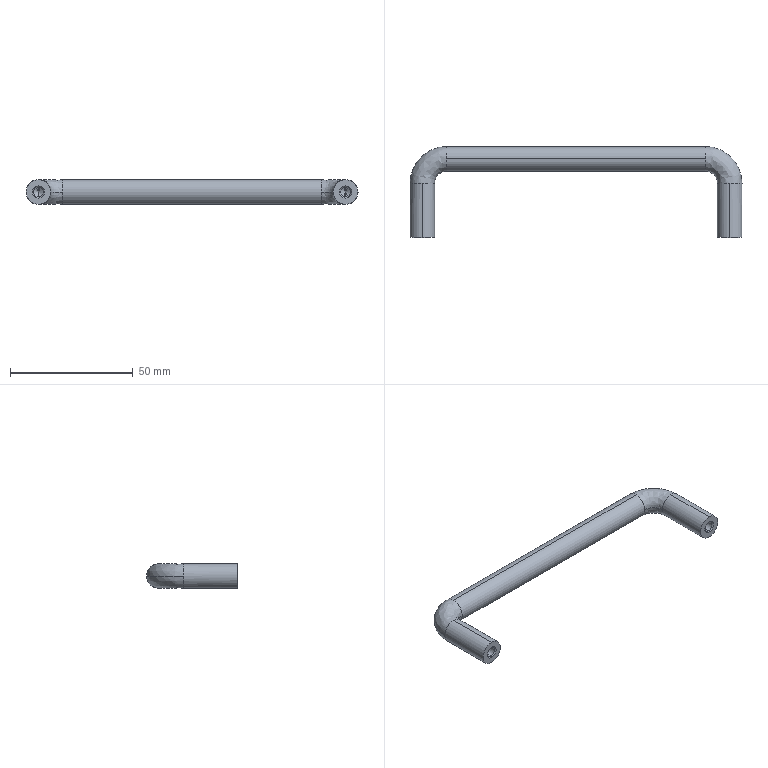Part | SolidWorks | features MBimport 1 | 1 solid | 24 faces | box 135 x 37 x 10 mm | volume 13834 mm3 | cylinder 10 | cone 8 | spline 4 | plane 2 | commonest cylinder face diameters 10 x6 4.134 x4
STEP:
#1=CARTESIAN_POINT('',(0.,13.193,0.));
#2=VERTEX_POINT('',#1);
#3=CARTESIAN_POINT('',(0.,12.,2.067));
#4=VERTEX_POINT('',#3);
#5=CARTESIAN_POINT('',(0.,12.,2.067));
#6=DIRECTION('',(0.,-0.5,0.866));
#7=VECTOR('',#6,1000.);
#8=LINE('',#5,#7);
#9=EDGE_CURVE('',#2,#4,#8,.T.);
#10=ORIENTED_EDGE('',*,*,#9,.F.);
#11=CARTESIAN_POINT('',(0.,12.,-2.067));
#12=VERTEX_POINT('',#11);
#13=CARTESIAN_POINT('',(0.,12.,-2.067));
#14=DIRECTION('',(0.,-0.5,-0.866));
#15=VECTOR('',#14,1000.);
#16=LINE('',#13,#15);
#17=EDGE_CURVE('',#2,#12,#16,.T.);
#18=ORIENTED_EDGE('',*,*,#17,.T.);
#19=CARTESIAN_POINT('',(0.,12.,0.));
#20=DIRECTION('',(0.,-1.,0.));
#21=DIRECTION('',(0.,0.,-1.));
#22=AXIS2_PLACEMENT_3D('',#19,#20,#21);
#23=CIRCLE('',#22,2.067);
#24=EDGE_CURVE('',#12,#4,#23,.T.);
#25=ORIENTED_EDGE('',*,*,#24,.T.);
#26=EDGE_LOOP('',(#10,#18,#25));
#27=FACE_OUTER_BOUND('',#26,.T.);
#28=CARTESIAN_POINT('',(0.,12.,0.));
#29=DIRECTION('',(0.,-1.,0.));
#30=DIRECTION('',(0.,0.,-1.));
#31=AXIS2_PLACEMENT_3D('',#28,#29,#30);
#32=CONICAL_SURFACE('',#31,2.067,1.047);
#33=ADVANCED_FACE('',(#27),#32,.F.);
#34=CARTESIAN_POINT('',(125.,13.193,0.));
#35=VERTEX_POINT('',#34);
#36=CARTESIAN_POINT('',(125.,12.,2.067));
#37=VERTEX_POINT('',#36);
#38=CARTESIAN_POINT('',(125.,12.,2.067));
#39=DIRECTION('',(0.,-0.5,0.866));
#40=VECTOR('',#39,1000.);
#41=LINE('',#38,#40);
#42=EDGE_CURVE('',#35,#37,#41,.T.);
#43=ORIENTED_EDGE('',*,*,#42,.F.);
#44=CARTESIAN_POINT('',(125.,12.,-2.067));
#45=VERTEX_POINT('',#44);
#46=CARTESIAN_POINT('',(125.,12.,-2.067));
#47=DIRECTION('',(0.,-0.5,-0.866));
#48=VECTOR('',#47,1000.);
#49=LINE('',#46,#48);
#50=EDGE_CURVE('',#35,#45,#49,.T.);
#51=ORIENTED_EDGE('',*,*,#50,.T.);
#52=CARTESIAN_POINT('',(125.,12.,0.));
#53=DIRECTION('',(0.,-1.,0.));
#54=DIRECTION('',(0.,0.,-1.));
#55=AXIS2_PLACEMENT_3D('',#52,#53,#54);
#56=CIRCLE('',#55,2.067);
#57=EDGE_CURVE('',#45,#37,#56,.T.);
#58=ORIENTED_EDGE('',*,*,#57,.T.);
#59=EDGE_LOOP('',(#43,#51,#58));
#60=FACE_OUTER_BOUND('',#59,.T.);
#61=CARTESIAN_POINT('',(125.,12.,0.));
#62=DIRECTION('',(0.,-1.,0.));
#63=DIRECTION('',(0.,0.,-1.));
#64=AXIS2_PLACEMENT_3D('',#61,#62,#63);
#65=CONICAL_SURFACE('',#64,2.067,1.047);
#66=ADVANCED_FACE('',(#60),#65,.F.);
#67=CARTESIAN_POINT('',(0.,0.433,2.067));
#68=VERTEX_POINT('',#67);
#69=CARTESIAN_POINT('',(0.,0.,2.067));
#70=DIRECTION('',(0.,-1.,0.));
#71=VECTOR('',#70,1000.);
#72=LINE('',#69,#71);
#73=EDGE_CURVE('',#4,#68,#72,.T.);
#74=ORIENTED_EDGE('',*,*,#73,.F.);
#75=ORIENTED_EDGE('',*,*,#24,.F.);
#76=CARTESIAN_POINT('',(0.,0.433,-2.067));
#77=VERTEX_POINT('',#76);
#78=CARTESIAN_POINT('',(0.,0.,-2.067));
#79=DIRECTION('',(0.,-1.,0.));
#80=VECTOR('',#79,1000.);
#81=LINE('',#78,#80);
#82=EDGE_CURVE('',#12,#77,#81,.T.);
#83=ORIENTED_EDGE('',*,*,#82,.T.);
#84=CARTESIAN_POINT('',(0.,0.433,0.));
#85=DIRECTION('',(0.,-1.,0.));
#86=DIRECTION('',(0.,0.,1.));
#87=AXIS2_PLACEMENT_3D('',#84,#85,#86);
#88=CIRCLE('',#87,2.067);
#89=EDGE_CURVE('',#77,#68,#88,.T.);
#90=ORIENTED_EDGE('',*,*,#89,.T.);
#91=EDGE_LOOP('',(#74,#75,#83,#90));
#92=FACE_OUTER_BOUND('',#91,.T.);
#93=CARTESIAN_POINT('',(0.,0.,0.));
#94=DIRECTION('',(0.,-1.,0.));
#95=DIRECTION('',(0.,0.,-1.));
#96=AXIS2_PLACEMENT_3D('',#93,#94,#95);
#97=CYLINDRICAL_SURFACE('',#96,2.067);
#98=ADVANCED_FACE('',(#92),#97,.F.);
#99=CARTESIAN_POINT('',(125.,0.433,2.067));
#100=VERTEX_POINT('',#99);
#101=CARTESIAN_POINT('',(125.,0.,2.067));
#102=DIRECTION('',(0.,-1.,0.));
#103=VECTOR('',#102,1000.);
#104=LINE('',#101,#103);
#105=EDGE_CURVE('',#37,#100,#104,.T.);
#106=ORIENTED_EDGE('',*,*,#105,.F.);
#107=ORIENTED_EDGE('',*,*,#57,.F.);
#108=CARTESIAN_POINT('',(125.,0.433,-2.067));
#109=VERTEX_POINT('',#108);
#110=CARTESIAN_POINT('',(125.,0.,-2.067));
#111=DIRECTION('',(0.,-1.,0.));
#112=VECTOR('',#111,1000.);
#113=LINE('',#110,#112);
#114=EDGE_CURVE('',#45,#109,#113,.T.);
#115=ORIENTED_EDGE('',*,*,#114,.T.);
#116=CARTESIAN_POINT('',(125.,0.433,0.));
#117=DIRECTION('',(0.,-1.,0.));
#118=DIRECTION('',(0.000000142,0.,1.));
#119=AXIS2_PLACEMENT_3D('',#116,#117,#118);
#120=CIRCLE('',#119,2.067);
#121=EDGE_CURVE('',#109,#100,#120,.T.);
#122=ORIENTED_EDGE('',*,*,#121,.T.);
#123=EDGE_LOOP('',(#106,#107,#115,#122));
#124=FACE_OUTER_BOUND('',#123,.T.);
#125=CARTESIAN_POINT('',(125.,0.,0.));
#126=DIRECTION('',(0.,-1.,0.));
#127=DIRECTION('',(0.,0.,-1.));
#128=AXIS2_PLACEMENT_3D('',#125,#126,#127);
#129=CYLINDRICAL_SURFACE('',#128,2.067);
#130=ADVANCED_FACE('',(#124),#129,.F.);
#131=CARTESIAN_POINT('',(0.,0.,2.5));
#132=VERTEX_POINT('',#131);
#133=CARTESIAN_POINT('',(0.,0.,2.5));
#134=DIRECTION('',(0.,-0.7071,0.7071));
#135=VECTOR('',#134,1000.);
#136=LINE('',#133,#135);
#137=EDGE_CURVE('',#68,#132,#136,.T.);
#138=ORIENTED_EDGE('',*,*,#137,.F.);
#139=ORIENTED_EDGE('',*,*,#89,.F.);
#140=CARTESIAN_POINT('',(0.,0.,-2.5));
#141=VERTEX_POINT('',#140);
#142=CARTESIAN_POINT('',(0.,0.,-2.5));
#143=DIRECTION('',(0.,-0.7071,-0.7071));
#144=VECTOR('',#143,1000.);
#145=LINE('',#142,#144);
#146=EDGE_CURVE('',#77,#141,#145,.T.);
#147=ORIENTED_EDGE('',*,*,#146,.T.);
#148=CARTESIAN_POINT('',(0.,0.,0.));
#149=DIRECTION('',(0.,1.,0.));
#150=DIRECTION('',(0.,0.,-1.));
#151=AXIS2_PLACEMENT_3D('',#148,#149,#150);
#152=CIRCLE('',#151,2.5);
#153=EDGE_CURVE('',#132,#141,#152,.T.);
#154=ORIENTED_EDGE('',*,*,#153,.F.);
#155=EDGE_LOOP('',(#138,#139,#147,#154));
#156=FACE_OUTER_BOUND('',#155,.T.);
#157=CARTESIAN_POINT('',(0.,0.,0.));
#158=DIRECTION('',(0.,-1.,0.));
#159=DIRECTION('',(0.,0.,-1.));
#160=AXIS2_PLACEMENT_3D('',#157,#158,#159);
#161=CONICAL_SURFACE('',#160,2.5,0.7854);
#162=ADVANCED_FACE('',(#156),#161,.F.);
#163=CARTESIAN_POINT('',(125.,0.,2.5));
#164=VERTEX_POINT('',#163);
#165=CARTESIAN_POINT('',(125.,0.,2.5));
#166=DIRECTION('',(0.,-0.7071,0.7071));
#167=VECTOR('',#166,1000.);
#168=LINE('',#165,#167);
#169=EDGE_CURVE('',#100,#164,#168,.T.);
#170=ORIENTED_EDGE('',*,*,#169,.F.);
#171=ORIENTED_EDGE('',*,*,#121,.F.);
#172=CARTESIAN_POINT('',(125.,0.,-2.5));
#173=VERTEX_POINT('',#172);
#174=CARTESIAN_POINT('',(125.,0.,-2.5));
#175=DIRECTION('',(0.,-0.7071,-0.7071));
#176=VECTOR('',#175,1000.);
#177=LINE('',#174,#176);
#178=EDGE_CURVE('',#109,#173,#177,.T.);
#179=ORIENTED_EDGE('',*,*,#178,.T.);
#180=CARTESIAN_POINT('',(125.,0.,0.));
#181=DIRECTION('',(0.,1.,0.));
#182=DIRECTION('',(0.,0.,-1.));
#183=AXIS2_PLACEMENT_3D('',#180,#181,#182);
#184=CIRCLE('',#183,2.5);
#185=EDGE_CURVE('',#164,#173,#184,.T.);
#186=ORIENTED_EDGE('',*,*,#185,.F.);
#187=EDGE_LOOP('',(#170,#171,#179,#186));
#188=FACE_OUTER_BOUND('',#187,.T.);
#189=CARTESIAN_POINT('',(125.,0.,0.));
#190=DIRECTION('',(0.,-1.,0.));
#191=DIRECTION('',(0.,0.,-1.));
#192=AXIS2_PLACEMENT_3D('',#189,#190,#191);
#193=CONICAL_SURFACE('',#192,2.5,0.7854);
#194=ADVANCED_FACE('',(#188),#193,.F.);
#195=CARTESIAN_POINT('',(0.,0.,0.));
#196=DIRECTION('',(0.,1.,0.));
#197=DIRECTION('',(0.,0.,-1.));
#198=AXIS2_PLACEMENT_3D('',#195,#196,#197);
#199=CIRCLE('',#198,2.5);
#200=EDGE_CURVE('',#141,#132,#199,.T.);
#201=ORIENTED_EDGE('',*,*,#200,.T.);
#202=ORIENTED_EDGE('',*,*,#153,.T.);
#203=EDGE_LOOP('',(#201,#202));
#204=FACE_BOUND('',#203,.T.);
#205=CARTESIAN_POINT('',(0.,0.,-5.));
#206=VERTEX_POINT('',#205);
#207=CARTESIAN_POINT('',(0.,0.,5.));
#208=VERTEX_POINT('',#207);
#209=CARTESIAN_POINT('',(0.,0.,0.));
#210=DIRECTION('',(0.,1.,0.));
#211=DIRECTION('',(0.,0.,-1.));
#212=AXIS2_PLACEMENT_3D('',#209,#210,#211);
#213=CIRCLE('',#212,5.);
#214=EDGE_CURVE('',#206,#208,#213,.T.);
#215=ORIENTED_EDGE('',*,*,#214,.F.);
#216=CARTESIAN_POINT('',(0.,0.,0.));
#217=DIRECTION('',(0.,1.,0.));
#218=DIRECTION('',(0.,0.,-1.));
#219=AXIS2_PLACEMENT_3D('',#216,#217,#218);
#220=CIRCLE('',#219,5.);
#221=EDGE_CURVE('',#208,#206,#220,.T.);
#222=ORIENTED_EDGE('',*,*,#221,.F.);
#223=EDGE_LOOP('',(#215,#222));
#224=FACE_OUTER_BOUND('',#223,.T.);
#225=CARTESIAN_POINT('',(-5.,0.,-5.));
#226=DIRECTION('',(0.,-1.,0.));
#227=DIRECTION('',(0.,0.,-1.));
#228=AXIS2_PLACEMENT_3D('',#225,#226,#227);
#229=PLANE('',#228);
#230=ADVANCED_FACE('',(#204,#224),#229,.T.);
#231=CARTESIAN_POINT('',(125.,0.,0.));
#232=DIRECTION('',(0.,1.,0.));
#233=DIRECTION('',(0.,0.,-1.));
#234=AXIS2_PLACEMENT_3D('',#231,#232,#233);
#235=CIRCLE('',#234,2.5);
#236=EDGE_CURVE('',#173,#164,#235,.T.);
#237=ORIENTED_EDGE('',*,*,#236,.T.);
#238=ORIENTED_EDGE('',*,*,#185,.T.);
#239=EDGE_LOOP('',(#237,#238));
#240=FACE_BOUND('',#239,.T.);
#241=CARTESIAN_POINT('',(125.,0.,-5.));
#242=VERTEX_POINT('',#241);
#243=CARTESIAN_POINT('',(125.,0.,5.));
#244=VERTEX_POINT('',#243);
#245=CARTESIAN_POINT('',(125.,0.,0.));
#246=DIRECTION('',(0.,1.,0.));
#247=DIRECTION('',(0.,0.,-1.));
#248=AXIS2_PLACEMENT_3D('',#245,#246,#247);
#249=CIRCLE('',#248,5.);
#250=EDGE_CURVE('',#242,#244,#249,.T.);
#251=ORIENTED_EDGE('',*,*,#250,.F.);
#252=CARTESIAN_POINT('',(125.,0.,0.));
#253=DIRECTION('',(0.,1.,0.));
#254=DIRECTION('',(0.,0.,-1.));
#255=AXIS2_PLACEMENT_3D('',#252,#253,#254);
#256=CIRCLE('',#255,5.);
#257=EDGE_CURVE('',#244,#242,#256,.T.);
#258=ORIENTED_EDGE('',*,*,#257,.F.);
#259=EDGE_LOOP('',(#251,#258));
#260=FACE_OUTER_BOUND('',#259,.T.);
#261=CARTESIAN_POINT('',(120.,0.,-5.));
#262=DIRECTION('',(0.,-1.,0.));
#263=DIRECTION('',(0.,0.,-1.));
#264=AXIS2_PLACEMENT_3D('',#261,#262,#263);
#265=PLANE('',#264);
#266=ADVANCED_FACE('',(#240,#260),#265,.T.);
#267=CARTESIAN_POINT('',(0.,22.,5.));
#268=VERTEX_POINT('',#267);
#269=CARTESIAN_POINT('',(0.,0.,5.));
#270=DIRECTION('',(0.,-1.,0.));
#271=VECTOR('',#270,1000.);
#272=LINE('',#269,#271);
#273=EDGE_CURVE('',#268,#208,#272,.T.);
#274=ORIENTED_EDGE('',*,*,#273,.F.);
#275=CARTESIAN_POINT('',(-5.,22.,0.));
#276=VERTEX_POINT('',#275);
#277=CARTESIAN_POINT('',(0.,22.,0.));
#278=DIRECTION('',(0.,1.,0.));
#279=DIRECTION('',(-1.,0.,0.));
#280=AXIS2_PLACEMENT_3D('',#277,#278,#279);
#281=CIRCLE('',#280,5.);
#282=EDGE_CURVE('',#276,#268,#281,.T.);
#283=ORIENTED_EDGE('',*,*,#282,.F.);
#284=CARTESIAN_POINT('',(0.,22.,-5.));
#285=VERTEX_POINT('',#284);
#286=CARTESIAN_POINT('',(0.,22.,0.));
#287=DIRECTION('',(0.,1.,0.));
#288=DIRECTION('',(-1.,0.,0.));
#289=AXIS2_PLACEMENT_3D('',#286,#287,#288);
#290=CIRCLE('',#289,5.);
#291=EDGE_CURVE('',#285,#276,#290,.T.);
#292=ORIENTED_EDGE('',*,*,#291,.F.);
#293=CARTESIAN_POINT('',(0.,0.,-5.));
#294=DIRECTION('',(0.,-1.,0.));
#295=VECTOR('',#294,1000.);
#296=LINE('',#293,#295);
#297=EDGE_CURVE('',#285,#206,#296,.T.);
#298=ORIENTED_EDGE('',*,*,#297,.T.);
#299=ORIENTED_EDGE('',*,*,#214,.T.);
#300=EDGE_LOOP('',(#274,#283,#292,#298,#299));
#301=FACE_OUTER_BOUND('',#300,.T.);
#302=CARTESIAN_POINT('',(0.,0.,0.));
#303=DIRECTION('',(0.,-1.,0.));
#304=DIRECTION('',(0.,0.,-1.));
#305=AXIS2_PLACEMENT_3D('',#302,#303,#304);
#306=CYLINDRICAL_SURFACE('',#305,5.);
#307=ADVANCED_FACE('',(#301),#306,.T.);
#308=CARTESIAN_POINT('',(125.,22.,5.));
#309=VERTEX_POINT('',#308);
#310=CARTESIAN_POINT('',(125.,0.,5.));
#311=DIRECTION('',(0.,-1.,0.));
#312=VECTOR('',#311,1000.);
#313=LINE('',#310,#312);
#314=EDGE_CURVE('',#309,#244,#313,.T.);
#315=ORIENTED_EDGE('',*,*,#314,.F.);
#316=CARTESIAN_POINT('',(120.,22.,0.));
#317=VERTEX_POINT('',#316);
#318=CARTESIAN_POINT('',(125.,22.,0.));
#319=DIRECTION('',(0.,1.,0.));
#320=DIRECTION('',(1.,0.,0.));
#321=AXIS2_PLACEMENT_3D('',#318,#319,#320);
#322=CIRCLE('',#321,5.);
#323=EDGE_CURVE('',#317,#309,#322,.T.);
#324=ORIENTED_EDGE('',*,*,#323,.F.);
#325=CARTESIAN_POINT('',(125.,22.,-5.));
#326=VERTEX_POINT('',#325);
#327=CARTESIAN_POINT('',(125.,22.,0.));
#328=DIRECTION('',(0.,1.,0.));
#329=DIRECTION('',(1.,0.,0.));
#330=AXIS2_PLACEMENT_3D('',#327,#328,#329);
#331=CIRCLE('',#330,5.);
#332=EDGE_CURVE('',#326,#317,#331,.T.);
#333=ORIENTED_EDGE('',*,*,#332,.F.);
#334=CARTESIAN_POINT('',(125.,0.,-5.));
#335=DIRECTION('',(0.,-1.,0.));
#336=VECTOR('',#335,1000.);
#337=LINE('',#334,#336);
#338=EDGE_CURVE('',#326,#242,#337,.T.);
#339=ORIENTED_EDGE('',*,*,#338,.T.);
#340=ORIENTED_EDGE('',*,*,#250,.T.);
#341=EDGE_LOOP('',(#315,#324,#333,#339,#340));
#342=FACE_OUTER_BOUND('',#341,.T.);
#343=CARTESIAN_POINT('',(125.,0.,0.));
#344=DIRECTION('',(0.,-1.,0.));
#345=DIRECTION('',(0.,0.,-1.));
#346=AXIS2_PLACEMENT_3D('',#343,#344,#345);
#347=CYLINDRICAL_SURFACE('',#346,5.);
#348=ADVANCED_FACE('',(#342),#347,.T.);
#349=CARTESIAN_POINT('',(5.,22.,0.));
#350=VERTEX_POINT('',#349);
#351=CARTESIAN_POINT('',(10.,27.,0.));
#352=VERTEX_POINT('',#351);
#353=CARTESIAN_POINT('',(10.,22.,0.));
#354=DIRECTION('',(0.,0.,-1.));
#355=DIRECTION('',(-1.,0.,0.));
#356=AXIS2_PLACEMENT_3D('',#353,#354,#355);
#357=CIRCLE('',#356,5.);
#358=EDGE_CURVE('',#350,#352,#357,.T.);
#359=ORIENTED_EDGE('',*,*,#358,.F.);
#360=CARTESIAN_POINT('',(0.,22.,0.));
#361=DIRECTION('',(0.,1.,0.));
#362=DIRECTION('',(-1.,0.,0.));
#363=AXIS2_PLACEMENT_3D('',#360,#361,#362);
#364=CIRCLE('',#363,5.);
#365=EDGE_CURVE('',#350,#285,#364,.T.);
#366=ORIENTED_EDGE('',*,*,#365,.T.);
#367=ORIENTED_EDGE('',*,*,#291,.T.);
#368=CARTESIAN_POINT('',(10.,37.,0.));
#369=VERTEX_POINT('',#368);
#370=CARTESIAN_POINT('',(10.,22.,0.));
#371=DIRECTION('',(0.,0.,-1.));
#372=DIRECTION('',(-1.,0.,0.));
#373=AXIS2_PLACEMENT_3D('',#370,#371,#372);
#374=CIRCLE('',#373,15.);
#375=EDGE_CURVE('',#276,#369,#374,.T.);
#376=ORIENTED_EDGE('',*,*,#375,.T.);
#377=CARTESIAN_POINT('',(10.,32.,-5.));
#378=VERTEX_POINT('',#377);
#379=CARTESIAN_POINT('',(10.,32.,0.));
#380=DIRECTION('',(1.,0.,0.));
#381=DIRECTION('',(0.,0.,-1.));
#382=AXIS2_PLACEMENT_3D('',#379,#380,#381);
#383=CIRCLE('',#382,5.);
#384=EDGE_CURVE('',#378,#369,#383,.T.);
#385=ORIENTED_EDGE('',*,*,#384,.F.);
#386=CARTESIAN_POINT('',(10.,32.,0.));
#387=DIRECTION('',(1.,0.,0.));
#388=DIRECTION('',(0.,0.,-1.));
#389=AXIS2_PLACEMENT_3D('',#386,#387,#388);
#390=CIRCLE('',#389,5.);
#391=EDGE_CURVE('',#352,#378,#390,.T.);
#392=ORIENTED_EDGE('',*,*,#391,.F.);
#393=EDGE_LOOP('',(#359,#366,#367,#376,#385,#392));
#394=FACE_OUTER_BOUND('',#393,.T.);
#395=CARTESIAN_POINT('',(5.,22.,0.));
#396=CARTESIAN_POINT('',(5.,24.929,0.));
#397=CARTESIAN_POINT('',(7.071,27.,0.));
#398=CARTESIAN_POINT('',(10.,27.,0.));
#399=CARTESIAN_POINT('',(5.,22.,-10.));
#400=CARTESIAN_POINT('',(5.,24.929,-10.));
#401=CARTESIAN_POINT('',(7.071,27.,-10.));
#402=CARTESIAN_POINT('',(10.,27.,-10.));
#403=CARTESIAN_POINT('',(-5.,22.,-10.));
#404=CARTESIAN_POINT('',(-5.,30.787,-10.));
#405=CARTESIAN_POINT('',(1.213,37.,-10.));
#406=CARTESIAN_POINT('',(10.,37.,-10.));
#407=CARTESIAN_POINT('',(-5.,22.,0.));
#408=CARTESIAN_POINT('',(-5.,30.787,0.));
#409=CARTESIAN_POINT('',(1.213,37.,0.));
#410=CARTESIAN_POINT('',(10.,37.,0.));
#411=(BOUNDED_SURFACE()B_SPLINE_SURFACE(3,3,((#395,#396,#397,#398),(#399,#400,#401,#402),(#403,#404,#405,#406),(#407,#408,#409,#410)),.UNSPECIFIED.,.F.,.F.,.F.)B_SPLINE_SURFACE_WITH_KNOTS((4,4),(4,4),(0.,1.),(0.,1.),.UNSPECIFIED.)GEOMETRIC_REPRESENTATION_ITEM()RATIONAL_B_SPLINE_SURFACE(((1.,0.8047,0.8047,1.),(0.3333,0.2682,0.2682,0.3333),(0.3333,0.2682,0.2682,0.3333),(1.,0.8047,0.8047,1.)))REPRESENTATION_ITEM('')SURFACE());
#412=ADVANCED_FACE('',(#394),#411,.T.);
#413=CARTESIAN_POINT('',(115.,27.,0.));
#414=VERTEX_POINT('',#413);
#415=CARTESIAN_POINT('',(115.,22.,0.));
#416=DIRECTION('',(0.,0.,1.));
#417=DIRECTION('',(1.,0.,0.));
#418=AXIS2_PLACEMENT_3D('',#415,#416,#417);
#419=CIRCLE('',#418,5.);
#420=EDGE_CURVE('',#317,#414,#419,.T.);
#421=ORIENTED_EDGE('',*,*,#420,.F.);
#422=ORIENTED_EDGE('',*,*,#323,.T.);
#423=CARTESIAN_POINT('',(130.,22.,0.));
#424=VERTEX_POINT('',#423);
#425=CARTESIAN_POINT('',(125.,22.,0.));
#426=DIRECTION('',(0.,1.,0.));
#427=DIRECTION('',(1.,0.,0.));
#428=AXIS2_PLACEMENT_3D('',#425,#426,#427);
#429=CIRCLE('',#428,5.);
#430=EDGE_CURVE('',#309,#424,#429,.T.);
#431=ORIENTED_EDGE('',*,*,#430,.T.);
#432=CARTESIAN_POINT('',(115.,37.,0.));
#433=VERTEX_POINT('',#432);
#434=CARTESIAN_POINT('',(115.,22.,0.));
#435=DIRECTION('',(0.,0.,1.));
#436=DIRECTION('',(1.,0.,0.));
#437=AXIS2_PLACEMENT_3D('',#434,#435,#436);
#438=CIRCLE('',#437,15.);
#439=EDGE_CURVE('',#424,#433,#438,.T.);
#440=ORIENTED_EDGE('',*,*,#439,.T.);
#441=CARTESIAN_POINT('',(115.,32.,5.));
#442=VERTEX_POINT('',#441);
#443=CARTESIAN_POINT('',(115.,32.,0.));
#444=DIRECTION('',(-1.,0.,0.));
#445=DIRECTION('',(0.,0.,-1.));
#446=AXIS2_PLACEMENT_3D('',#443,#444,#445);
#447=CIRCLE('',#446,5.);
#448=EDGE_CURVE('',#442,#433,#447,.T.);
#449=ORIENTED_EDGE('',*,*,#448,.F.);
#450=CARTESIAN_POINT('',(115.,32.,0.));
#451=DIRECTION('',(-1.,0.,0.));
#452=DIRECTION('',(0.,0.,-1.));
#453=AXIS2_PLACEMENT_3D('',#450,#451,#452);
#454=CIRCLE('',#453,5.);
#455=EDGE_CURVE('',#414,#442,#454,.T.);
#456=ORIENTED_EDGE('',*,*,#455,.F.);
#457=EDGE_LOOP('',(#421,#422,#431,#440,#449,#456));
#458=FACE_OUTER_BOUND('',#457,.T.);
#459=CARTESIAN_POINT('',(120.,22.,0.));
#460=CARTESIAN_POINT('',(120.,24.929,0.));
#461=CARTESIAN_POINT('',(117.929,27.,0.));
#462=CARTESIAN_POINT('',(115.,27.,0.));
#463=CARTESIAN_POINT('',(120.,22.,10.));
#464=CARTESIAN_POINT('',(120.,24.929,10.));
#465=CARTESIAN_POINT('',(117.929,27.,10.));
#466=CARTESIAN_POINT('',(115.,27.,10.));
#467=CARTESIAN_POINT('',(130.,22.,10.));
#468=CARTESIAN_POINT('',(130.,30.787,10.));
#469=CARTESIAN_POINT('',(123.787,37.,10.));
#470=CARTESIAN_POINT('',(115.,37.,10.));
#471=CARTESIAN_POINT('',(130.,22.,0.));
#472=CARTESIAN_POINT('',(130.,30.787,0.));
#473=CARTESIAN_POINT('',(123.787,37.,0.));
#474=CARTESIAN_POINT('',(115.,37.,0.));
#475=(BOUNDED_SURFACE()B_SPLINE_SURFACE(3,3,((#459,#460,#461,#462),(#463,#464,#465,#466),(#467,#468,#469,#470),(#471,#472,#473,#474)),.UNSPECIFIED.,.F.,.F.,.F.)B_SPLINE_SURFACE_WITH_KNOTS((4,4),(4,4),(0.,1.),(0.,1.),.UNSPECIFIED.)GEOMETRIC_REPRESENTATION_ITEM()RATIONAL_B_SPLINE_SURFACE(((1.,0.8047,0.8047,1.),(0.3333,0.2682,0.2682,0.3333),(0.3333,0.2682,0.2682,0.3333),(1.,0.8047,0.8047,1.)))REPRESENTATION_ITEM('')SURFACE());
#476=ADVANCED_FACE('',(#458),#475,.T.);
#477=CARTESIAN_POINT('',(10.,32.,5.));
#478=VERTEX_POINT('',#477);
#479=CARTESIAN_POINT('',(70.,32.,5.));
#480=DIRECTION('',(1.,0.,0.));
#481=VECTOR('',#480,1000.);
#482=LINE('',#479,#481);
#483=EDGE_CURVE('',#478,#442,#482,.T.);
#484=ORIENTED_EDGE('',*,*,#483,.F.);
#485=CARTESIAN_POINT('',(10.,32.,0.));
#486=DIRECTION('',(1.,0.,0.));
#487=DIRECTION('',(0.,0.,-1.));
#488=AXIS2_PLACEMENT_3D('',#485,#486,#487);
#489=CIRCLE('',#488,5.);
#490=EDGE_CURVE('',#478,#352,#489,.T.);
#491=ORIENTED_EDGE('',*,*,#490,.T.);
#492=ORIENTED_EDGE('',*,*,#391,.T.);
#493=CARTESIAN_POINT('',(115.,32.,-5.));
#494=VERTEX_POINT('',#493);
#495=CARTESIAN_POINT('',(70.,32.,-5.));
#496=DIRECTION('',(1.,0.,0.));
#497=VECTOR('',#496,1000.);
#498=LINE('',#495,#497);
#499=EDGE_CURVE('',#378,#494,#498,.T.);
#500=ORIENTED_EDGE('',*,*,#499,.T.);
#501=CARTESIAN_POINT('',(115.,32.,0.));
#502=DIRECTION('',(-1.,0.,0.));
#503=DIRECTION('',(0.,0.,-1.));
#504=AXIS2_PLACEMENT_3D('',#501,#502,#503);
#505=CIRCLE('',#504,5.);
#506=EDGE_CURVE('',#494,#414,#505,.T.);
#507=ORIENTED_EDGE('',*,*,#506,.T.);
#508=ORIENTED_EDGE('',*,*,#455,.T.);
#509=EDGE_LOOP('',(#484,#491,#492,#500,#507,#508));
#510=FACE_OUTER_BOUND('',#509,.T.);
#511=CARTESIAN_POINT('',(70.,32.,0.));
#512=DIRECTION('',(1.,0.,0.));
#513=DIRECTION('',(0.,0.,-1.));
#514=AXIS2_PLACEMENT_3D('',#511,#512,#513);
#515=CYLINDRICAL_SURFACE('',#514,5.);
#516=ADVANCED_FACE('',(#510),#515,.T.);
#517=ORIENTED_EDGE('',*,*,#17,.F.);
#518=ORIENTED_EDGE('',*,*,#9,.T.);
#519=CARTESIAN_POINT('',(0.,12.,0.));
#520=DIRECTION('',(0.,-1.,0.));
#521=DIRECTION('',(0.,0.,-1.));
#522=AXIS2_PLACEMENT_3D('',#519,#520,#521);
#523=CIRCLE('',#522,2.067);
#524=EDGE_CURVE('',#4,#12,#523,.T.);
#525=ORIENTED_EDGE('',*,*,#524,.T.);
#526=EDGE_LOOP('',(#517,#518,#525));
#527=FACE_OUTER_BOUND('',#526,.T.);
#528=CARTESIAN_POINT('',(0.,12.,0.));
#529=DIRECTION('',(0.,-1.,0.));
#530=DIRECTION('',(0.,0.,-1.));
#531=AXIS2_PLACEMENT_3D('',#528,#529,#530);
#532=CONICAL_SURFACE('',#531,2.067,1.047);
#533=ADVANCED_FACE('',(#527),#532,.F.);
#534=ORIENTED_EDGE('',*,*,#50,.F.);
#535=ORIENTED_EDGE('',*,*,#42,.T.);
#536=CARTESIAN_POINT('',(125.,12.,0.));
#537=DIRECTION('',(0.,-1.,0.));
#538=DIRECTION('',(0.,0.,-1.));
#539=AXIS2_PLACEMENT_3D('',#536,#537,#538);
#540=CIRCLE('',#539,2.067);
#541=EDGE_CURVE('',#37,#45,#540,.T.);
#542=ORIENTED_EDGE('',*,*,#541,.T.);
#543=EDGE_LOOP('',(#534,#535,#542));
#544=FACE_OUTER_BOUND('',#543,.T.);
#545=CARTESIAN_POINT('',(125.,12.,0.));
#546=DIRECTION('',(0.,-1.,0.));
#547=DIRECTION('',(0.,0.,-1.));
#548=AXIS2_PLACEMENT_3D('',#545,#546,#547);
#549=CONICAL_SURFACE('',#548,2.067,1.047);
#550=ADVANCED_FACE('',(#544),#549,.F.);
#551=ORIENTED_EDGE('',*,*,#524,.F.);
#552=ORIENTED_EDGE('',*,*,#73,.T.);
#553=CARTESIAN_POINT('',(0.,0.433,0.));
#554=DIRECTION('',(0.,-1.,0.));
#555=DIRECTION('',(0.,0.,1.));
#556=AXIS2_PLACEMENT_3D('',#553,#554,#555);
#557=CIRCLE('',#556,2.067);
#558=EDGE_CURVE('',#68,#77,#557,.T.);
#559=ORIENTED_EDGE('',*,*,#558,.T.);
#560=ORIENTED_EDGE('',*,*,#82,.F.);
#561=EDGE_LOOP('',(#551,#552,#559,#560));
#562=FACE_OUTER_BOUND('',#561,.T.);
#563=CARTESIAN_POINT('',(0.,0.,0.));
#564=DIRECTION('',(0.,-1.,0.));
#565=DIRECTION('',(0.,0.,-1.));
#566=AXIS2_PLACEMENT_3D('',#563,#564,#565);
#567=CYLINDRICAL_SURFACE('',#566,2.067);
#568=ADVANCED_FACE('',(#562),#567,.F.);
#569=ORIENTED_EDGE('',*,*,#541,.F.);
#570=ORIENTED_EDGE('',*,*,#105,.T.);
#571=CARTESIAN_POINT('',(125.,0.433,0.));
#572=DIRECTION('',(0.,-1.,0.));
#573=DIRECTION('',(0.000000142,0.,1.));
#574=AXIS2_PLACEMENT_3D('',#571,#572,#573);
#575=CIRCLE('',#574,2.067);
#576=EDGE_CURVE('',#100,#109,#575,.T.);
#577=ORIENTED_EDGE('',*,*,#576,.T.);
#578=ORIENTED_EDGE('',*,*,#114,.F.);
#579=EDGE_LOOP('',(#569,#570,#577,#578));
#580=FACE_OUTER_BOUND('',#579,.T.);
#581=CARTESIAN_POINT('',(125.,0.,0.));
#582=DIRECTION('',(0.,-1.,0.));
#583=DIRECTION('',(0.,0.,-1.));
#584=AXIS2_PLACEMENT_3D('',#581,#582,#583);
#585=CYLINDRICAL_SURFACE('',#584,2.067);
#586=ADVANCED_FACE('',(#580),#585,.F.);
#587=ORIENTED_EDGE('',*,*,#558,.F.);
#588=ORIENTED_EDGE('',*,*,#137,.T.);
#589=ORIENTED_EDGE('',*,*,#200,.F.);
#590=ORIENTED_EDGE('',*,*,#146,.F.);
#591=EDGE_LOOP('',(#587,#588,#589,#590));
#592=FACE_OUTER_BOUND('',#591,.T.);
#593=CARTESIAN_POINT('',(0.,0.,0.));
#594=DIRECTION('',(0.,-1.,0.));
#595=DIRECTION('',(0.,0.,-1.));
#596=AXIS2_PLACEMENT_3D('',#593,#594,#595);
#597=CONICAL_SURFACE('',#596,2.5,0.7854);
#598=ADVANCED_FACE('',(#592),#597,.F.);
#599=ORIENTED_EDGE('',*,*,#576,.F.);
#600=ORIENTED_EDGE('',*,*,#169,.T.);
#601=ORIENTED_EDGE('',*,*,#236,.F.);
#602=ORIENTED_EDGE('',*,*,#178,.F.);
#603=EDGE_LOOP('',(#599,#600,#601,#602));
#604=FACE_OUTER_BOUND('',#603,.T.);
#605=CARTESIAN_POINT('',(125.,0.,0.));
#606=DIRECTION('',(0.,-1.,0.));
#607=DIRECTION('',(0.,0.,-1.));
#608=AXIS2_PLACEMENT_3D('',#605,#606,#607);
#609=CONICAL_SURFACE('',#608,2.5,0.7854);
#610=ADVANCED_FACE('',(#604),#609,.F.);
#611=CARTESIAN_POINT('',(0.,22.,0.));
#612=DIRECTION('',(0.,1.,0.));
#613=DIRECTION('',(-1.,0.,0.));
#614=AXIS2_PLACEMENT_3D('',#611,#612,#613);
#615=CIRCLE('',#614,5.);
#616=EDGE_CURVE('',#268,#350,#615,.T.);
#617=ORIENTED_EDGE('',*,*,#616,.F.);
#618=ORIENTED_EDGE('',*,*,#273,.T.);
#619=ORIENTED_EDGE('',*,*,#221,.T.);
#620=ORIENTED_EDGE('',*,*,#297,.F.);
#621=ORIENTED_EDGE('',*,*,#365,.F.);
#622=EDGE_LOOP('',(#617,#618,#619,#620,#621));
#623=FACE_OUTER_BOUND('',#622,.T.);
#624=CARTESIAN_POINT('',(0.,0.,0.));
#625=DIRECTION('',(0.,-1.,0.));
#626=DIRECTION('',(0.,0.,-1.));
#627=AXIS2_PLACEMENT_3D('',#624,#625,#626);
#628=CYLINDRICAL_SURFACE('',#627,5.);
#629=ADVANCED_FACE('',(#623),#628,.T.);
#630=ORIENTED_EDGE('',*,*,#430,.F.);
#631=ORIENTED_EDGE('',*,*,#314,.T.);
#632=ORIENTED_EDGE('',*,*,#257,.T.);
#633=ORIENTED_EDGE('',*,*,#338,.F.);
#634=CARTESIAN_POINT('',(125.,22.,0.));
#635=DIRECTION('',(0.,1.,0.));
#636=DIRECTION('',(1.,0.,0.));
#637=AXIS2_PLACEMENT_3D('',#634,#635,#636);
#638=CIRCLE('',#637,5.);
#639=EDGE_CURVE('',#424,#326,#638,.T.);
#640=ORIENTED_EDGE('',*,*,#639,.F.);
#641=EDGE_LOOP('',(#630,#631,#632,#633,#640));
#642=FACE_OUTER_BOUND('',#641,.T.);
#643=CARTESIAN_POINT('',(125.,0.,0.));
#644=DIRECTION('',(0.,-1.,0.));
#645=DIRECTION('',(0.,0.,-1.));
#646=AXIS2_PLACEMENT_3D('',#643,#644,#645);
#647=CYLINDRICAL_SURFACE('',#646,5.);
#648=ADVANCED_FACE('',(#642),#647,.T.);
#649=ORIENTED_EDGE('',*,*,#616,.T.);
#650=ORIENTED_EDGE('',*,*,#358,.T.);
#651=ORIENTED_EDGE('',*,*,#490,.F.);
#652=CARTESIAN_POINT('',(10.,32.,0.));
#653=DIRECTION('',(1.,0.,0.));
#654=DIRECTION('',(0.,0.,-1.));
#655=AXIS2_PLACEMENT_3D('',#652,#653,#654);
#656=CIRCLE('',#655,5.);
#657=EDGE_CURVE('',#369,#478,#656,.T.);
#658=ORIENTED_EDGE('',*,*,#657,.F.);
#659=ORIENTED_EDGE('',*,*,#375,.F.);
#660=ORIENTED_EDGE('',*,*,#282,.T.);
#661=EDGE_LOOP('',(#649,#650,#651,#658,#659,#660));
#662=FACE_OUTER_BOUND('',#661,.T.);
#663=CARTESIAN_POINT('',(-5.,22.,0.));
#664=CARTESIAN_POINT('',(-5.,30.787,0.));
#665=CARTESIAN_POINT('',(1.213,37.,0.));
#666=CARTESIAN_POINT('',(10.,37.,0.));
#667=CARTESIAN_POINT('',(-5.,22.,10.));
#668=CARTESIAN_POINT('',(-5.,30.787,10.));
#669=CARTESIAN_POINT('',(1.213,37.,10.));
#670=CARTESIAN_POINT('',(10.,37.,10.));
#671=CARTESIAN_POINT('',(5.,22.,10.));
#672=CARTESIAN_POINT('',(5.,24.929,10.));
#673=CARTESIAN_POINT('',(7.071,27.,10.));
#674=CARTESIAN_POINT('',(10.,27.,10.));
#675=CARTESIAN_POINT('',(5.,22.,0.));
#676=CARTESIAN_POINT('',(5.,24.929,0.));
#677=CARTESIAN_POINT('',(7.071,27.,0.));
#678=CARTESIAN_POINT('',(10.,27.,0.));
#679=(BOUNDED_SURFACE()B_SPLINE_SURFACE(3,3,((#663,#664,#665,#666),(#667,#668,#669,#670),(#671,#672,#673,#674),(#675,#676,#677,#678)),.UNSPECIFIED.,.F.,.F.,.T.)B_SPLINE_SURFACE_WITH_KNOTS((4,4),(4,4),(0.,1.),(0.,1.),.UNSPECIFIED.)GEOMETRIC_REPRESENTATION_ITEM()RATIONAL_B_SPLINE_SURFACE(((1.,0.8047,0.8047,1.),(0.3333,0.2682,0.2682,0.3333),(0.3333,0.2682,0.2682,0.3333),(1.,0.8047,0.8047,1.)))REPRESENTATION_ITEM('')SURFACE());
#680=ADVANCED_FACE('',(#662),#679,.T.);
#681=ORIENTED_EDGE('',*,*,#332,.T.);
#682=ORIENTED_EDGE('',*,*,#420,.T.);
#683=ORIENTED_EDGE('',*,*,#506,.F.);
#684=CARTESIAN_POINT('',(115.,32.,0.));
#685=DIRECTION('',(-1.,0.,0.));
#686=DIRECTION('',(0.,0.,-1.));
#687=AXIS2_PLACEMENT_3D('',#684,#685,#686);
#688=CIRCLE('',#687,5.);
#689=EDGE_CURVE('',#433,#494,#688,.T.);
#690=ORIENTED_EDGE('',*,*,#689,.F.);
#691=ORIENTED_EDGE('',*,*,#439,.F.);
#692=ORIENTED_EDGE('',*,*,#639,.T.);
#693=EDGE_LOOP('',(#681,#682,#683,#690,#691,#692));
#694=FACE_OUTER_BOUND('',#693,.T.);
#695=CARTESIAN_POINT('',(130.,22.,0.));
#696=CARTESIAN_POINT('',(130.,30.787,0.));
#697=CARTESIAN_POINT('',(123.787,37.,0.));
#698=CARTESIAN_POINT('',(115.,37.,0.));
#699=CARTESIAN_POINT('',(130.,22.,-10.));
#700=CARTESIAN_POINT('',(130.,30.787,-10.));
#701=CARTESIAN_POINT('',(123.787,37.,-10.));
#702=CARTESIAN_POINT('',(115.,37.,-10.));
#703=CARTESIAN_POINT('',(120.,22.,-10.));
#704=CARTESIAN_POINT('',(120.,24.929,-10.));
#705=CARTESIAN_POINT('',(117.929,27.,-10.));
#706=CARTESIAN_POINT('',(115.,27.,-10.));
#707=CARTESIAN_POINT('',(120.,22.,0.));
#708=CARTESIAN_POINT('',(120.,24.929,0.));
#709=CARTESIAN_POINT('',(117.929,27.,0.));
#710=CARTESIAN_POINT('',(115.,27.,0.));
#711=(BOUNDED_SURFACE()B_SPLINE_SURFACE(3,3,((#695,#696,#697,#698),(#699,#700,#701,#702),(#703,#704,#705,#706),(#707,#708,#709,#710)),.UNSPECIFIED.,.F.,.F.,.T.)B_SPLINE_SURFACE_WITH_KNOTS((4,4),(4,4),(0.,1.),(0.,1.),.UNSPECIFIED.)GEOMETRIC_REPRESENTATION_ITEM()RATIONAL_B_SPLINE_SURFACE(((1.,0.8047,0.8047,1.),(0.3333,0.2682,0.2682,0.3333),(0.3333,0.2682,0.2682,0.3333),(1.,0.8047,0.8047,1.)))REPRESENTATION_ITEM('')SURFACE());
#712=ADVANCED_FACE('',(#694),#711,.T.);
#713=ORIENTED_EDGE('',*,*,#657,.T.);
#714=ORIENTED_EDGE('',*,*,#483,.T.);
#715=ORIENTED_EDGE('',*,*,#448,.T.);
#716=ORIENTED_EDGE('',*,*,#689,.T.);
#717=ORIENTED_EDGE('',*,*,#499,.F.);
#718=ORIENTED_EDGE('',*,*,#384,.T.);
#719=EDGE_LOOP('',(#713,#714,#715,#716,#717,#718));
#720=FACE_OUTER_BOUND('',#719,.T.);
#721=CARTESIAN_POINT('',(70.,32.,0.));
#722=DIRECTION('',(1.,0.,0.));
#723=DIRECTION('',(0.,0.,-1.));
#724=AXIS2_PLACEMENT_3D('',#721,#722,#723);
#725=CYLINDRICAL_SURFACE('',#724,5.);
#726=ADVANCED_FACE('',(#720),#725,.T.);
#727=CLOSED_SHELL('',(#33,#66,#98,#130,#162,#194,#230,#266,#307,#348,#412,#476,#516,#533,#550,#568,#586,#598,#610,#629,#648,#680,#712,#726));
#728=MANIFOLD_SOLID_BREP('',#727);
#729=CARTESIAN_POINT('',(0.,0.,0.));
#730=DIRECTION('',(0.,0.,1.));
#731=DIRECTION('',(1.,0.,0.));
#732=AXIS2_PLACEMENT_3D('',#729,#730,#731);
#733=(LENGTH_UNIT()NAMED_UNIT(*)SI_UNIT(.MILLI.,.METRE.));
#734=UNCERTAINTY_MEASURE_WITH_UNIT(LENGTH_MEASURE(0.00001),#733,'','');
#735=(NAMED_UNIT(*)PLANE_ANGLE_UNIT()SI_UNIT($,.RADIAN.));
#736=(NAMED_UNIT(*)SI_UNIT($,.STERADIAN.)SOLID_ANGLE_UNIT());
#737=(GEOMETRIC_REPRESENTATION_CONTEXT(3)GLOBAL_UNCERTAINTY_ASSIGNED_CONTEXT((#734))GLOBAL_UNIT_ASSIGNED_CONTEXT((#733,#735,#736))REPRESENTATION_CONTEXT('',''));
#738=ADVANCED_BREP_SHAPE_REPRESENTATION('',(#728,#732),#737);